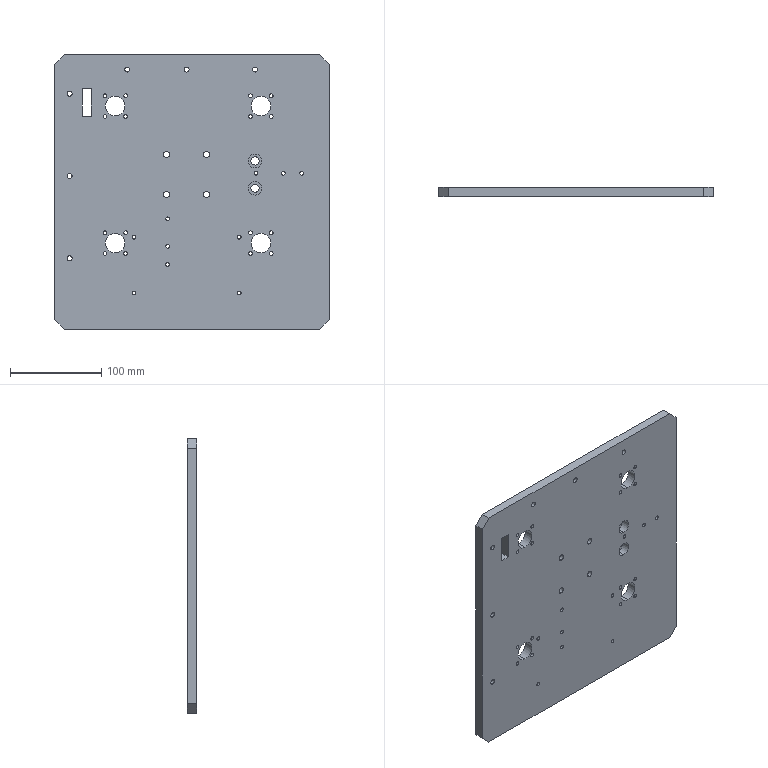Part | SolidWorks | features HoleWzd 6, Cut 3, Chamfer 1, Extrusion 1 | 1 solid | 125 faces | box 300 x 10 x 300 mm | volume 864543 mm3 | cylinder 102 | plane 23 | commonest cylinder face diameters 4.2 x52 5.5 x12 10 x12 6.8 x8 21.5 x8 9 x4